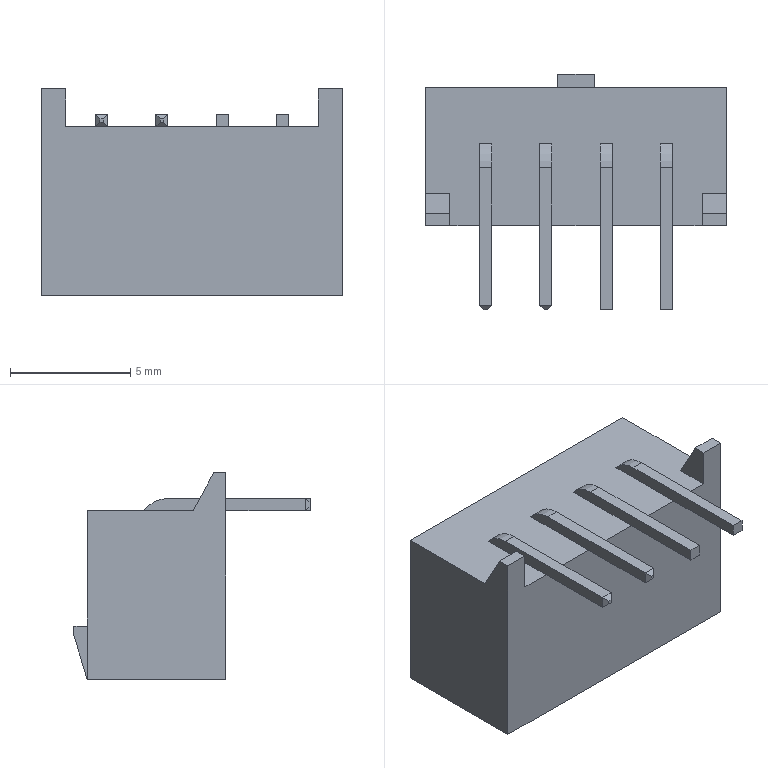Part | STEP file | 12M0-U000-0002_A2512WRO-4P_1 | 1 solid | 101 faces | box 12.48 x 9.8 x 8.57 mm | volume 221.308 mm3 | plane 93 | cylinder 8 | commonest cylinder face diameters 0.5 x4 2.5 x4